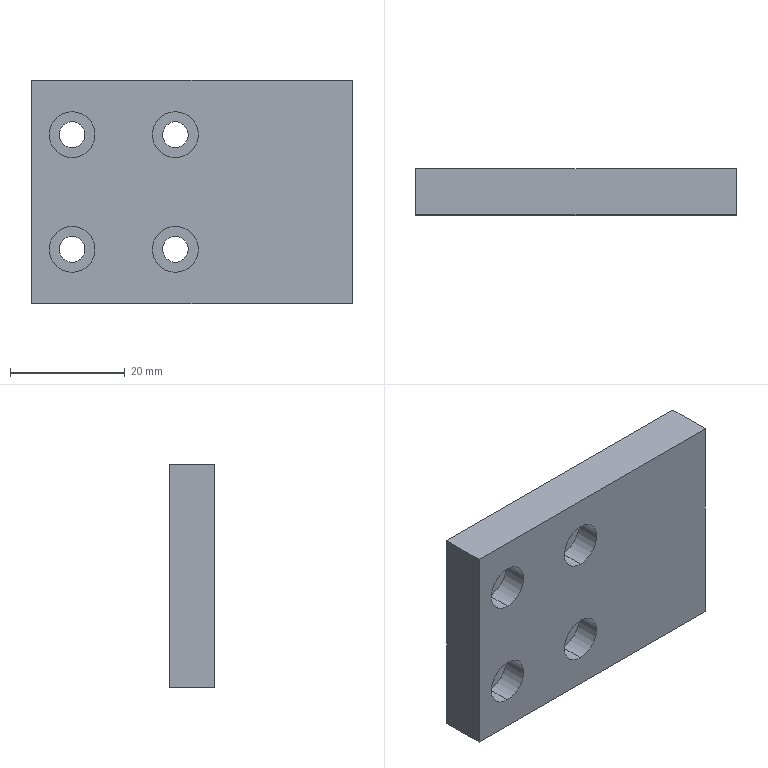Part | STEP file | ASND-0110-TPIM-067 | 1 solid | 38 faces | box 55.8 x 8 x 39 mm | volume 15980 mm3 | cylinder 22 | plane 10 | cone 6 | commonest cylinder face diameters 4.5 x8 8 x8 3.3 x6